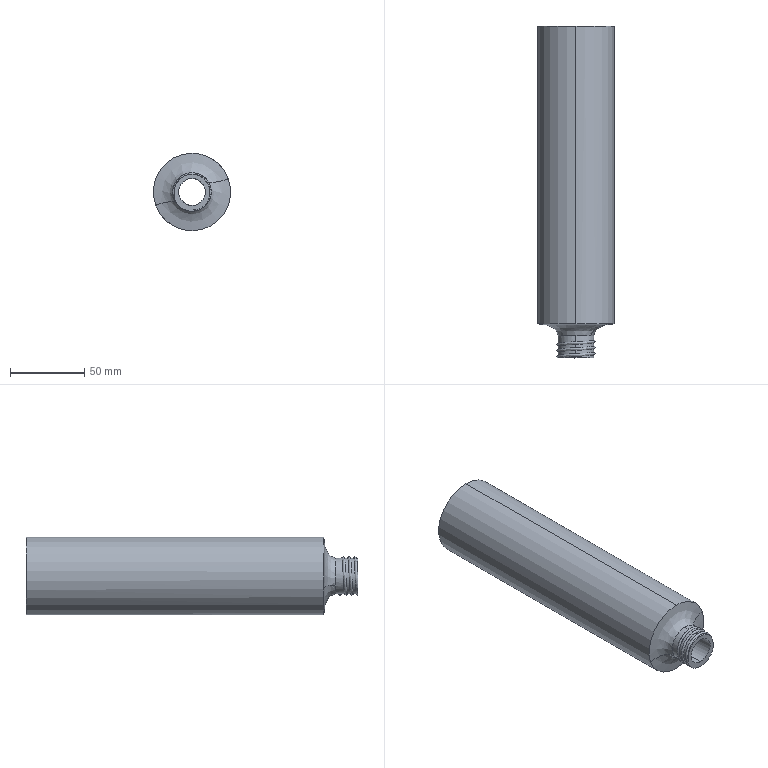Part | SolidWorks | features Blend 1, Helix 1, ICE 1, Revolution 1, Shell 1, Sweep 1 | 1 solid | 24 faces | box 52.001 x 224.797 x 52 mm | volume 100616 mm3 | cylinder 14 | spline 7 | plane 3 | commonest cylinder face diameters 24 x8 18 x2 46 x2 52 x2